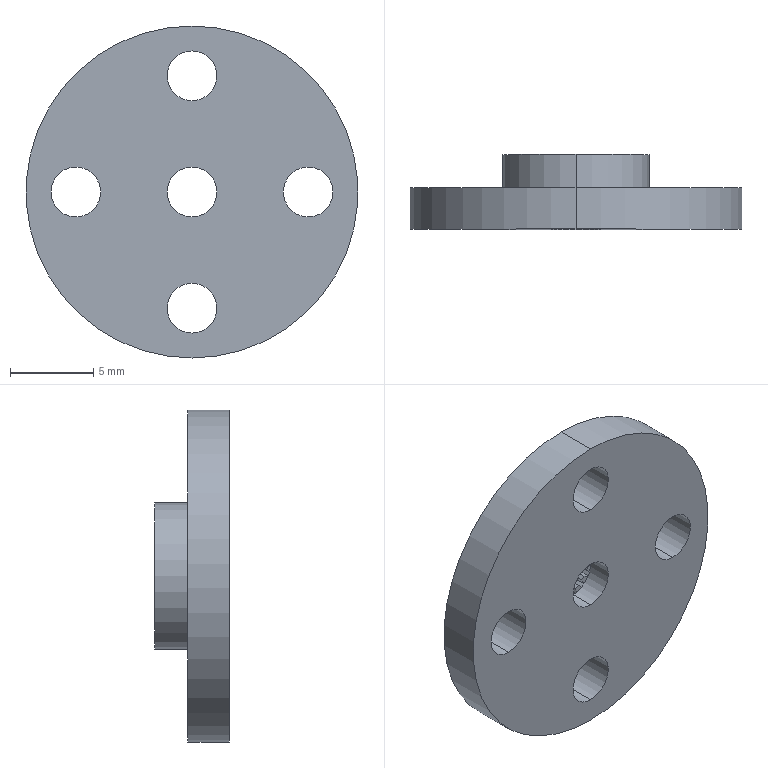Part | STEP file | Metal main rudder disc | 1 solid | 116 faces | box 20 x 4.5 x 20 mm | volume 750.526 mm3 | plane 100 | cylinder 16 | commonest cylinder face diameters 3 x10 6 x2 8.8 x2 20 x2